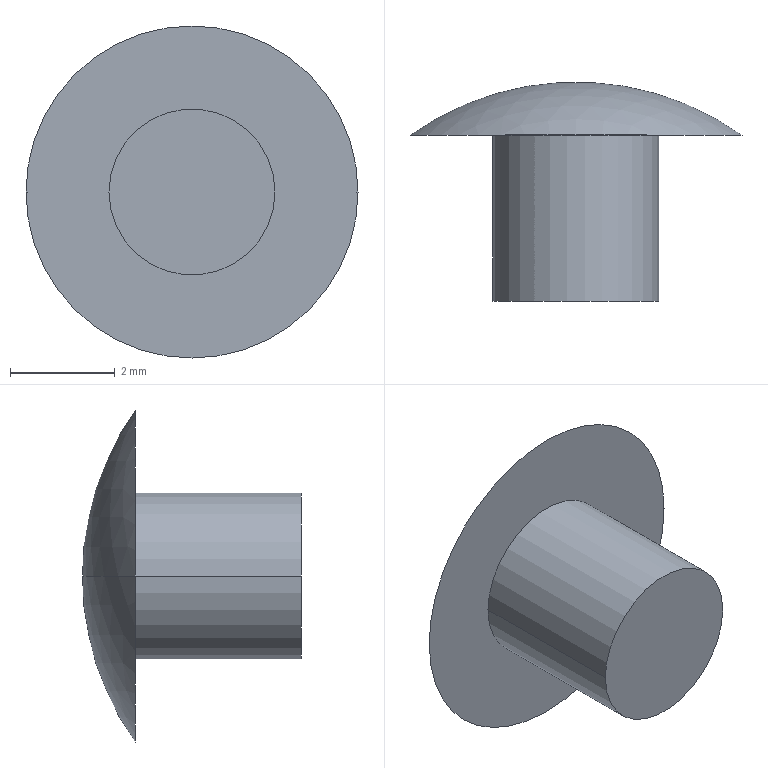Part | NX | features BREP 1 | 1 solid | 6 faces | box 6.35 x 4.191 x 6.35 mm | volume 41.774 mm3 | plane 2 | sphere 2 | cylinder 2 | commonest cylinder face diameters 3.175 x2
STEP:
#1=CARTESIAN_POINT('',(-3.175,0.,0.));
#2=VERTEX_POINT('',#1);
#3=CARTESIAN_POINT('',(3.175,0.,0.));
#4=VERTEX_POINT('',#3);
#5=CARTESIAN_POINT('',(0.,0.,0.));
#6=DIRECTION('',(0.,1.,0.));
#7=DIRECTION('',(-1.,0.,0.));
#8=AXIS2_PLACEMENT_3D('',#5,#6,#7);
#9=CIRCLE('',#8,3.175);
#10=EDGE_CURVE('',#2,#4,#9,.T.);
#11=ORIENTED_EDGE('',*,*,#10,.F.);
#12=CARTESIAN_POINT('',(0.,0.,0.));
#13=DIRECTION('',(0.,-1.,0.));
#14=DIRECTION('',(-1.,0.,0.));
#15=AXIS2_PLACEMENT_3D('',#12,#13,#14);
#16=CIRCLE('',#15,3.175);
#17=EDGE_CURVE('',#2,#4,#16,.T.);
#18=ORIENTED_EDGE('',*,*,#17,.T.);
#19=EDGE_LOOP('',(#11,#18));
#20=FACE_BOUND('',#19,.T.);
#21=CARTESIAN_POINT('',(-1.587,0.,0.));
#22=VERTEX_POINT('',#21);
#23=CARTESIAN_POINT('',(1.587,0.,0.));
#24=VERTEX_POINT('',#23);
#25=CARTESIAN_POINT('',(0.,0.,0.));
#26=DIRECTION('',(0.,-1.,0.));
#27=DIRECTION('',(-1.,0.,0.));
#28=AXIS2_PLACEMENT_3D('',#25,#26,#27);
#29=CIRCLE('',#28,1.587);
#30=EDGE_CURVE('',#22,#24,#29,.T.);
#31=ORIENTED_EDGE('',*,*,#30,.F.);
#32=CARTESIAN_POINT('',(0.,0.,0.));
#33=DIRECTION('',(0.,1.,0.));
#34=DIRECTION('',(-1.,0.,0.));
#35=AXIS2_PLACEMENT_3D('',#32,#33,#34);
#36=CIRCLE('',#35,1.587);
#37=EDGE_CURVE('',#22,#24,#36,.T.);
#38=ORIENTED_EDGE('',*,*,#37,.T.);
#39=EDGE_LOOP('',(#31,#38));
#40=FACE_BOUND('',#39,.T.);
#41=CARTESIAN_POINT('',(0.,0.,0.));
#42=DIRECTION('',(0.,-1.,0.));
#43=DIRECTION('',(0.,0.,-1.));
#44=AXIS2_PLACEMENT_3D('',#41,#42,#43);
#45=PLANE('',#44);
#46=ADVANCED_FACE('',(#20,#40),#45,.T.);
#47=CARTESIAN_POINT('',(0.,-4.453,0.));
#48=DIRECTION('',(0.,0.,1.));
#49=DIRECTION('',(0.5806,0.8142,0.));
#50=AXIS2_PLACEMENT_3D('',#47,#48,#49);
#51=CIRCLE('',#50,5.469);
#52=EDGE_CURVE('',#4,#2,#51,.T.);
#53=ORIENTED_EDGE('',*,*,#52,.F.);
#54=ORIENTED_EDGE('',*,*,#17,.F.);
#55=EDGE_LOOP('',(#53,#54));
#56=FACE_BOUND('',#55,.T.);
#57=CARTESIAN_POINT('',(0.,-4.453,0.));
#58=DIRECTION('',(0.,0.,1.));
#59=DIRECTION('',(1.,0.,0.));
#60=AXIS2_PLACEMENT_3D('',#57,#58,#59);
#61=SPHERICAL_SURFACE('',#60,5.469);
#62=ADVANCED_FACE('',(#56),#61,.T.);
#63=ORIENTED_EDGE('',*,*,#10,.T.);
#64=ORIENTED_EDGE('',*,*,#52,.T.);
#65=EDGE_LOOP('',(#63,#64));
#66=FACE_BOUND('',#65,.T.);
#67=CARTESIAN_POINT('',(0.,-4.453,0.));
#68=DIRECTION('',(0.,0.,1.));
#69=DIRECTION('',(1.,0.,0.));
#70=AXIS2_PLACEMENT_3D('',#67,#68,#69);
#71=SPHERICAL_SURFACE('',#70,5.469);
#72=ADVANCED_FACE('',(#66),#71,.T.);
#73=CARTESIAN_POINT('',(-1.587,-3.175,0.));
#74=VERTEX_POINT('',#73);
#75=CARTESIAN_POINT('',(1.587,-3.175,0.));
#76=VERTEX_POINT('',#75);
#77=CARTESIAN_POINT('',(0.,-3.175,0.));
#78=DIRECTION('',(0.,1.,0.));
#79=DIRECTION('',(-1.,0.,0.));
#80=AXIS2_PLACEMENT_3D('',#77,#78,#79);
#81=CIRCLE('',#80,1.587);
#82=EDGE_CURVE('',#74,#76,#81,.T.);
#83=ORIENTED_EDGE('',*,*,#82,.T.);
#84=CARTESIAN_POINT('',(1.587,-3.175,0.));
#85=DIRECTION('',(0.,1.,0.));
#86=VECTOR('',#85,1000.);
#87=LINE('',#84,#86);
#88=EDGE_CURVE('',#76,#24,#87,.T.);
#89=ORIENTED_EDGE('',*,*,#88,.T.);
#90=ORIENTED_EDGE('',*,*,#37,.F.);
#91=CARTESIAN_POINT('',(-1.587,-3.175,0.));
#92=DIRECTION('',(0.,1.,0.));
#93=VECTOR('',#92,1000.);
#94=LINE('',#91,#93);
#95=EDGE_CURVE('',#74,#22,#94,.T.);
#96=ORIENTED_EDGE('',*,*,#95,.F.);
#97=EDGE_LOOP('',(#83,#89,#90,#96));
#98=FACE_BOUND('',#97,.T.);
#99=CARTESIAN_POINT('',(0.,1.226,0.));
#100=DIRECTION('',(0.,-1.,0.));
#101=DIRECTION('',(1.,0.,0.));
#102=AXIS2_PLACEMENT_3D('',#99,#100,#101);
#103=CYLINDRICAL_SURFACE('',#102,1.587);
#104=ADVANCED_FACE('',(#98),#103,.T.);
#105=ORIENTED_EDGE('',*,*,#30,.T.);
#106=ORIENTED_EDGE('',*,*,#88,.F.);
#107=CARTESIAN_POINT('',(0.,-3.175,0.));
#108=DIRECTION('',(0.,-1.,0.));
#109=DIRECTION('',(-1.,0.,0.));
#110=AXIS2_PLACEMENT_3D('',#107,#108,#109);
#111=CIRCLE('',#110,1.587);
#112=EDGE_CURVE('',#74,#76,#111,.T.);
#113=ORIENTED_EDGE('',*,*,#112,.F.);
#114=ORIENTED_EDGE('',*,*,#95,.T.);
#115=EDGE_LOOP('',(#105,#106,#113,#114));
#116=FACE_BOUND('',#115,.T.);
#117=CARTESIAN_POINT('',(0.,1.226,0.));
#118=DIRECTION('',(0.,-1.,0.));
#119=DIRECTION('',(1.,0.,0.));
#120=AXIS2_PLACEMENT_3D('',#117,#118,#119);
#121=CYLINDRICAL_SURFACE('',#120,1.587);
#122=ADVANCED_FACE('',(#116),#121,.T.);
#123=ORIENTED_EDGE('',*,*,#112,.T.);
#124=ORIENTED_EDGE('',*,*,#82,.F.);
#125=EDGE_LOOP('',(#123,#124));
#126=FACE_BOUND('',#125,.T.);
#127=CARTESIAN_POINT('',(0.,-3.175,0.));
#128=DIRECTION('',(0.,-1.,0.));
#129=DIRECTION('',(0.,0.,-1.));
#130=AXIS2_PLACEMENT_3D('',#127,#128,#129);
#131=PLANE('',#130);
#132=ADVANCED_FACE('',(#126),#131,.T.);
#133=CLOSED_SHELL('',(#46,#62,#72,#104,#122,#132));
#134=MANIFOLD_SOLID_BREP('',#133);
#135=(LENGTH_UNIT()NAMED_UNIT(*)SI_UNIT(.MILLI.,.METRE.));
#136=UNCERTAINTY_MEASURE_WITH_UNIT(LENGTH_MEASURE(0.00001),#135,'','');
#137=(NAMED_UNIT(*)PLANE_ANGLE_UNIT()SI_UNIT($,.RADIAN.));
#138=(NAMED_UNIT(*)SI_UNIT($,.STERADIAN.)SOLID_ANGLE_UNIT());
#139=(GEOMETRIC_REPRESENTATION_CONTEXT(3)GLOBAL_UNCERTAINTY_ASSIGNED_CONTEXT((#136))GLOBAL_UNIT_ASSIGNED_CONTEXT((#135,#137,#138))REPRESENTATION_CONTEXT('',''));
#140=ADVANCED_BREP_SHAPE_REPRESENTATION('',(#134),#139);